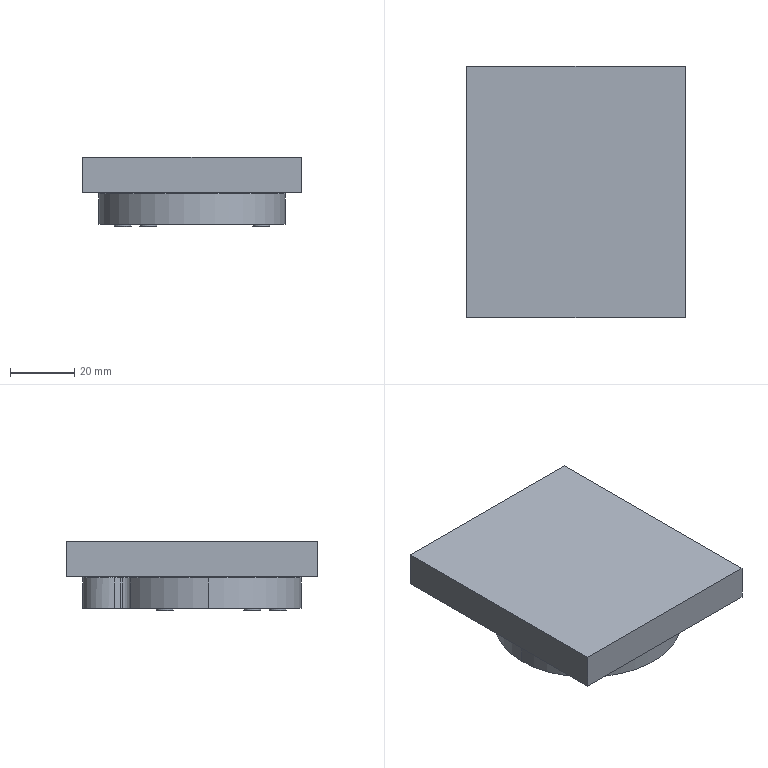NC program | NX | posted with a generic post | part box 68 x 78.27 x 21.8 mm
Lines 751 to 1704 of 10371:
(CAVITY_MILL_COPY_COPY , TOOL : D4)
N1488 T11 M6
N1490 G54
N1492 G17 G0 G90 X-13.811 Y15.944 S9500 M3
N1494 G43 Z30. H11
N1496 Z-0.7
N1498 G94 G1 Z-1.2 F1000.
N1500 X-14.149 Y16.097
N1502 G3 X-15.145 Y15.999 R1.
N1504 X-16.092 Y15.287 R26. F2000.
N1506 G2 X-16.209 Y14.361 R2.5
N1508 G3 X-16.001 Y13.383 R1.
N1510 G1 X-15.879 Y13.247
N1512 Z-0.7
N1514 G0 X-13.811 Y15.944 Z-1.1
N1516 G1 Z-1.6 F1000.
N1518 X-14.149 Y16.097
N1520 G3 X-15.145 Y15.999 R1.
N1522 X-16.092 Y15.287 R26. F2000.
N1524 G2 X-16.209 Y14.361 R2.5
N1526 G3 X-16.001 Y13.383 R1.
N1528 G1 X-15.879 Y13.247
N1530 Z-1.1
N1532 G0 X-13.811 Y15.944 Z-1.5
N1534 G1 Z-2. F1000.
N1536 X-14.149 Y16.097
N1538 G3 X-15.145 Y15.999 R1.
N1540 X-16.092 Y15.287 R26. F2000.
N1542 G2 X-16.209 Y14.361 R2.5
N1544 G3 X-16.001 Y13.383 R1.
N1546 G1 X-15.879 Y13.247
N1548 Z-1.5
N1550 G0 X-13.811 Y15.944 Z-1.9
N1552 G1 Z-2.4 F1000.
N1554 X-14.149 Y16.097
N1556 G3 X-15.145 Y15.999 R1.
N1558 X-16.092 Y15.287 R26. F2000.
N1560 G2 X-16.209 Y14.361 R2.5
N1562 G3 X-16.001 Y13.383 R1.
N1564 G1 X-15.879 Y13.247
N1566 Z-1.9
N1568 G0 X-13.811 Y15.944 Z-2.3
N1570 G1 Z-2.8 F1000.
N1572 X-14.149 Y16.097
N1574 G3 X-15.145 Y15.999 R1.
N1576 X-16.092 Y15.287 R26. F2000.
N1578 G2 X-16.209 Y14.361 R2.5
N1580 G3 X-16.001 Y13.383 R1.
N1582 G1 X-15.879 Y13.247
N1584 Z-2.3
N1586 G0 X-13.811 Y15.944 Z-2.7
N1588 G1 Z-3.2 F1000.
N1590 X-14.149 Y16.097
N1592 G3 X-15.145 Y15.999 R1.
N1594 X-16.092 Y15.287 R26. F2000.
N1596 G2 X-16.209 Y14.361 R2.5
N1598 G3 X-16.001 Y13.383 R1.
N1600 G1 X-15.879 Y13.247
N1602 Z-2.7
N1604 G0 X-13.811 Y15.944 Z-3.1
N1606 G1 Z-3.6 F1000.
N1608 X-14.149 Y16.097
N1610 G3 X-15.145 Y15.999 R1.
N1612 X-16.092 Y15.287 R26. F2000.
N1614 G2 X-16.209 Y14.361 R2.5
N1616 G3 X-16.001 Y13.383 R1.
N1618 G1 X-15.879 Y13.247
N1620 Z-3.1
N1622 G0 X-13.811 Y15.944 Z-3.5
N1624 G1 Z-4. F1000.
N1626 X-14.149 Y16.097
N1628 G3 X-15.145 Y15.999 R1.
N1630 X-16.092 Y15.287 R26. F2000.
N1632 G2 X-16.209 Y14.361 R2.5
N1634 G3 X-16.001 Y13.383 R1.
N1636 G1 X-15.879 Y13.247
N1638 Z-3.5
N1640 G0 X-13.811 Y15.944 Z-3.9
N1642 G1 Z-4.4 F1000.
N1644 X-14.149 Y16.097
N1646 G3 X-15.145 Y15.999 R1.
N1648 X-16.092 Y15.287 R26. F2000.
N1650 G2 X-16.209 Y14.361 R2.5
N1652 G3 X-16.001 Y13.383 R1.
N1654 G1 X-15.879 Y13.247
N1656 Z-3.9
N1658 G0 X-13.811 Y15.944 Z-4.3
N1660 G1 Z-4.8 F1000.
N1662 X-14.149 Y16.097
N1664 G3 X-15.145 Y15.999 R1.
N1666 X-16.092 Y15.287 R26. F2000.
N1668 G2 X-16.209 Y14.361 R2.5
N1670 G3 X-16.001 Y13.383 R1.
N1672 G1 X-15.879 Y13.247
N1674 Z-4.3
N1676 G0 X-13.811 Y15.944 Z-4.7
N1678 G1 Z-5.2 F1000.
N1680 X-14.149 Y16.097
N1682 G3 X-15.145 Y15.999 R1.
N1684 X-16.092 Y15.287 R26. F2000.
N1686 G2 X-16.209 Y14.361 R2.5
N1688 G3 X-16.001 Y13.383 R1.
N1690 G1 X-15.879 Y13.247
N1692 Z-4.7
N1694 G0 X-13.811 Y15.944 Z-5.1
N1696 G1 Z-5.6 F1000.
N1698 X-14.149 Y16.097
N1700 G3 X-15.145 Y15.999 R1.
N1702 X-16.092 Y15.287 R26. F2000.
N1704 G2 X-16.209 Y14.361 R2.5
N1706 G3 X-16.001 Y13.383 R1.
N1708 G1 X-15.879 Y13.247
N1710 Z-5.1
N1712 G0 X-13.811 Y15.944 Z-5.5
N1714 G1 Z-6. F1000.
N1716 X-14.149 Y16.097
N1718 G3 X-15.145 Y15.999 R1.
N1720 X-16.092 Y15.287 R26. F2000.
N1722 G2 X-16.209 Y14.361 R2.5
N1724 G3 X-16.001 Y13.383 R1.
N1726 G1 X-15.879 Y13.247
N1728 Z-5.5
N1730 G0 X-13.811 Y15.944 Z-5.9
N1732 G1 Z-6.4 F1000.
N1734 X-14.149 Y16.097
N1736 G3 X-15.145 Y15.999 R1.
N1738 X-16.092 Y15.287 R26. F2000.
N1740 G2 X-16.209 Y14.361 R2.5
N1742 G3 X-16.001 Y13.383 R1.
N1744 G1 X-15.879 Y13.247
N1746 Z-5.9
N1748 G0 X-13.811 Y15.944 Z-6.3
N1750 G1 Z-6.8 F1000.
N1752 X-14.149 Y16.097
N1754 G3 X-15.145 Y15.999 R1.
N1756 X-16.092 Y15.287 R26. F2000.
N1758 G2 X-16.209 Y14.361 R2.5
N1760 G3 X-16.001 Y13.383 R1.
N1762 G1 X-15.879 Y13.247
N1764 Z-6.3
N1766 G0 X-13.811 Y15.944 Z-6.7
N1768 G1 Z-7.2 F1000.
N1770 X-14.149 Y16.097
N1772 G3 X-15.145 Y15.999 R1.
N1774 X-16.092 Y15.287 R26. F2000.
N1776 G2 X-16.209 Y14.361 R2.5
N1778 G3 X-16.001 Y13.383 R1.
N1780 G1 X-15.879 Y13.247
N1782 Z-6.7
N1784 G0 X-13.811 Y15.944 Z-7.1
N1786 G1 Z-7.6 F1000.
N1788 X-14.149 Y16.097
N1790 G3 X-15.145 Y15.999 R1.
N1792 X-16.092 Y15.287 R26. F2000.
N1794 G2 X-16.209 Y14.361 R2.5
N1796 G3 X-16.001 Y13.383 R1.
N1798 G1 X-15.879 Y13.247
N1800 Z-7.1
N1802 G0 X-13.811 Y15.944 Z-7.5
N1804 G1 Z-8. F1000.
N1806 X-14.149 Y16.097
N1808 G3 X-15.145 Y15.999 R1.
N1810 X-16.092 Y15.287 R26. F2000.
N1812 G2 X-16.209 Y14.361 R2.5
N1814 G3 X-16.001 Y13.383 R1.
N1816 G1 X-15.879 Y13.247
N1818 Z-7.5
N1820 G0 X-13.811 Y15.944 Z-7.9
N1822 G1 Z-8.4 F1000.
N1824 X-14.149 Y16.097
N1826 G3 X-15.145 Y15.999 R1.
N1828 X-16.092 Y15.287 R26. F2000.
N1830 G2 X-16.209 Y14.361 R2.5
N1832 G3 X-16.001 Y13.383 R1.
N1834 G1 X-15.879 Y13.247
N1836 Z-7.9
N1838 G0 X-13.811 Y15.944 Z-8.3
N1840 G1 Z-8.8 F1000.
N1842 X-14.149 Y16.097
N1844 G3 X-15.145 Y15.999 R1.
N1846 X-16.092 Y15.287 R26. F2000.
N1848 G2 X-16.209 Y14.361 R2.5
N1850 G3 X-16.001 Y13.383 R1.
N1852 G1 X-15.879 Y13.247
N1854 Z-8.3
N1856 G0 X-12.092 Y16.975 Z-8.633
N1858 G1 Z-9.133 F1000.
N1860 X-12.417 Y17.154
N1862 G3 X-13.417 Y17.136 R1.
N1864 X-15.863 Y15.465 R26. F2000.
N1866 G1 X-14.342 Y13.096
N1868 G3 X-13.453 Y12.637 R1.
N1870 G1 X-13.107 Y12.654
N1872 Z-8.633
N1874 G0 X-12.092 Y16.975 Z-8.967
N1876 G1 Z-9.467 F1000.
N1878 X-12.417 Y17.154
N1880 G3 X-13.417 Y17.136 R1.
N1882 X-15.863 Y15.465 R26. F2000.
N1884 G1 X-14.342 Y13.096
N1886 G3 X-13.453 Y12.637 R1.
N1888 G1 X-13.107 Y12.654
N1890 Z-8.967
N1892 G0 X-12.092 Y16.975 Z-9.3
N1894 G1 Z-9.8 F1000.
N1896 X-12.417 Y17.154
N1898 G3 X-13.417 Y17.136 R1.
N1900 X-15.863 Y15.465 R26. F2000.
N1902 G1 X-14.342 Y13.096
N1904 G3 X-13.453 Y12.637 R1.
N1906 G1 X-13.107 Y12.654
N1908 Z-9.3
N1910 G0 Z-5.8
N1912 X-10.957 Y9.306
N1914 Z-8.633
N1916 G1 Z-9.133 F1000.
N1918 X-11.116 Y8.998
N1920 G3 X-11.069 Y7.999 R1.
N1922 G1 X-9.482 Y5.528 F2000.
N1924 X-7.032 Y7.148
N1926 G3 X-6.585 Y8.042 R1.
N1928 G1 X-6.606 Y8.388
N1930 Z-8.633
N1932 G0 X-10.957 Y9.306 Z-8.967
N1934 G1 Z-9.467 F1000.
N1936 X-11.116 Y8.998
N1938 G3 X-11.069 Y7.999 R1.
N1940 G1 X-9.482 Y5.528 F2000.
N1942 X-7.032 Y7.148
N1944 G3 X-6.585 Y8.042 R1.
N1946 G1 X-6.606 Y8.388
N1948 Z-8.967
N1950 G0 X-10.957 Y9.306 Z-9.3
N1952 G1 Z-9.8 F1000.
N1954 X-11.116 Y8.998
N1956 G3 X-11.069 Y7.999 R1.
N1958 G1 X-9.482 Y5.528 F2000.
N1960 X-7.032 Y7.148
N1962 G3 X-6.585 Y8.042 R1.
N1964 G1 X-6.606 Y8.388
N1966 Z-9.3
N1968 G0 Z30.
N1970 X2.622 Y23.856
N1972 Z-0.7
N1974 G1 Z-1.2 F1000.
N1976 X2.46 Y23.94
N1978 G3 X1.461 Y23.895 R1.
N1980 G2 X0.853 Y23.614 R2.5 F2000.
N1982 X0.471 Y23.021 R6.
N1984 G3 X0.363 Y22.027 R1.
N1986 G1 X0.468 Y21.788
N1988 Z-0.7
N1990 G0 X2.622 Y23.856 Z-1.1
N1992 G1 Z-1.6 F1000.
N1994 X2.46 Y23.94
N1996 G3 X1.461 Y23.895 R1.
N1998 G2 X0.853 Y23.614 R2.5 F2000.
N2000 X0.471 Y23.021 R6.
N2002 G3 X0.363 Y22.027 R1.
N2004 G1 X0.468 Y21.788
N2006 Z-1.1
N2008 G0 X2.622 Y23.856 Z-1.5
N2010 G1 Z-2. F1000.
N2012 X2.46 Y23.94
N2014 G3 X1.461 Y23.895 R1.
N2016 G2 X0.853 Y23.614 R2.5 F2000.
N2018 X0.471 Y23.021 R6.
N2020 G3 X0.363 Y22.027 R1.
N2022 G1 X0.468 Y21.788
N2024 Z-1.5
N2026 G0 X2.622 Y23.856 Z-1.9
N2028 G1 Z-2.4 F1000.
N2030 X2.46 Y23.94
N2032 G3 X1.461 Y23.895 R1.
N2034 G2 X0.853 Y23.614 R2.5 F2000.
N2036 X0.471 Y23.021 R6.
N2038 G3 X0.363 Y22.027 R1.
N2040 G1 X0.468 Y21.788
N2042 Z-1.9
N2044 G0 X2.622 Y23.856 Z-2.3
N2046 G1 Z-2.8 F1000.
N2048 X2.46 Y23.94
N2050 G3 X1.461 Y23.895 R1.
N2052 G2 X0.853 Y23.614 R2.5 F2000.
N2054 X0.471 Y23.021 R6.
N2056 G3 X0.363 Y22.027 R1.
N2058 G1 X0.468 Y21.788
N2060 Z-2.3
N2062 G0 X2.622 Y23.856 Z-2.7
N2064 G1 Z-3.2 F1000.
N2066 X2.46 Y23.94
N2068 G3 X1.461 Y23.895 R1.
N2070 G2 X0.853 Y23.614 R2.5 F2000.
N2072 X0.471 Y23.021 R6.
N2074 G3 X0.363 Y22.027 R1.
N2076 G1 X0.468 Y21.788
N2078 Z-2.7
N2080 G0 X2.622 Y23.856 Z-3.1
N2082 G1 Z-3.6 F1000.
N2084 X2.46 Y23.94
N2086 G3 X1.461 Y23.895 R1.
N2088 G2 X0.853 Y23.614 R2.5 F2000.
N2090 X0.471 Y23.021 R6.
N2092 G3 X0.363 Y22.027 R1.
N2094 G1 X0.468 Y21.788
N2096 Z-3.1
N2098 G0 X2.622 Y23.856 Z-3.5
N2100 G1 Z-4. F1000.
N2102 X2.46 Y23.94
N2104 G3 X1.461 Y23.895 R1.
N2106 G2 X0.853 Y23.614 R2.5 F2000.
N2108 X0.471 Y23.021 R6.
N2110 G3 X0.363 Y22.027 R1.
N2112 G1 X0.468 Y21.788
N2114 Z-3.5
N2116 G0 X2.622 Y23.856 Z-3.9
N2118 G1 Z-4.4 F1000.
N2120 X2.46 Y23.94
N2122 G3 X1.461 Y23.895 R1.
N2124 G2 X0.853 Y23.614 R2.5 F2000.
N2126 X0.471 Y23.021 R6.
N2128 G3 X0.363 Y22.027 R1.
N2130 G1 X0.468 Y21.788
N2132 Z-3.9
N2134 G0 X2.622 Y23.856 Z-4.3
N2136 G1 Z-4.8 F1000.
N2138 X2.46 Y23.94
N2140 G3 X1.461 Y23.895 R1.
N2142 G2 X0.853 Y23.614 R2.5 F2000.
N2144 X0.471 Y23.021 R6.
N2146 G3 X0.363 Y22.027 R1.
N2148 G1 X0.468 Y21.788
N2150 Z-4.3
N2152 G0 X2.622 Y23.856 Z-4.7
N2154 G1 Z-5.2 F1000.
N2156 X2.46 Y23.94
N2158 G3 X1.461 Y23.895 R1.
N2160 G2 X0.853 Y23.614 R2.5 F2000.
N2162 X0.471 Y23.021 R6.
N2164 G3 X0.363 Y22.027 R1.
N2166 G1 X0.468 Y21.788
N2168 Z-4.7
N2170 G0 X2.622 Y23.856 Z-5.1
N2172 G1 Z-5.6 F1000.
N2174 X2.46 Y23.94
N2176 G3 X1.461 Y23.895 R1.
N2178 G2 X0.853 Y23.614 R2.5 F2000.
N2180 X0.471 Y23.021 R6.
N2182 G3 X0.363 Y22.027 R1.
N2184 G1 X0.468 Y21.788
N2186 Z-5.1
N2188 G0 X2.622 Y23.856 Z-5.5
N2190 G1 Z-6. F1000.
N2192 X2.46 Y23.94
N2194 G3 X1.461 Y23.895 R1.
N2196 G2 X0.853 Y23.614 R2.5 F2000.
N2198 X0.471 Y23.021 R6.
N2200 G3 X0.363 Y22.027 R1.
N2202 G1 X0.468 Y21.788
N2204 Z-5.5
N2206 G0 X2.622 Y23.856 Z-5.9
N2208 G1 Z-6.4 F1000.
N2210 X2.46 Y23.94
N2212 G3 X1.461 Y23.895 R1.
N2214 G2 X0.853 Y23.614 R2.5 F2000.
N2216 X0.471 Y23.021 R6.
N2218 G3 X0.363 Y22.027 R1.
N2220 G1 X0.468 Y21.788
N2222 Z-5.9
N2224 G0 X2.622 Y23.856 Z-6.3
N2226 G1 Z-6.8 F1000.
N2228 X2.46 Y23.94
N2230 G3 X1.461 Y23.895 R1.
N2232 G2 X0.853 Y23.614 R2.5 F2000.
N2234 X0.471 Y23.021 R6.
N2236 G3 X0.363 Y22.027 R1.
N2238 G1 X0.468 Y21.788
N2240 Z-6.3
N2242 G0 X2.622 Y23.856 Z-6.7
N2244 G1 Z-7.2 F1000.
N2246 X2.46 Y23.94
N2248 G3 X1.461 Y23.895 R1.
N2250 G2 X0.853 Y23.614 R2.5 F2000.
N2252 X0.471 Y23.021 R6.
N2254 G3 X0.363 Y22.027 R1.
N2256 G1 X0.468 Y21.788
N2258 Z-6.7
N2260 G0 X2.622 Y23.856 Z-7.1
N2262 G1 Z-7.6 F1000.
N2264 X2.46 Y23.94
N2266 G3 X1.461 Y23.895 R1.
N2268 G2 X0.853 Y23.614 R2.5 F2000.
N2270 X0.471 Y23.021 R6.
N2272 G3 X0.363 Y22.027 R1.
N2274 G1 X0.468 Y21.788
N2276 Z-7.1
N2278 G0 X2.622 Y23.856 Z-7.5
N2280 G1 Z-8. F1000.
N2282 X2.46 Y23.94
N2284 G3 X1.461 Y23.895 R1.
N2286 G2 X0.853 Y23.614 R2.5 F2000.
N2288 X0.471 Y23.021 R6.
N2290 G3 X0.363 Y22.027 R1.
N2292 G1 X0.468 Y21.788
N2294 Z-7.5
N2296 G0 X2.622 Y23.856 Z-7.9
N2298 G1 Z-8.4 F1000.
N2300 X2.46 Y23.94
N2302 G3 X1.461 Y23.895 R1.
N2304 G2 X0.853 Y23.614 R2.5 F2000.
N2306 X0.471 Y23.021 R6.
N2308 G3 X0.363 Y22.027 R1.
N2310 G1 X0.468 Y21.788
N2312 Z-7.9
N2314 G0 X2.622 Y23.856 Z-8.3
N2316 G1 Z-8.8 F1000.
N2318 X2.46 Y23.94
N2320 G3 X1.461 Y23.895 R1.
N2322 G2 X0.853 Y23.614 R2.5 F2000.
N2324 X0.471 Y23.021 R6.
N2326 G3 X0.363 Y22.027 R1.
N2328 G1 X0.468 Y21.788
N2330 Z-8.3
N2332 G0 X3.225 Y21.978 Z-8.633
N2334 G1 Z-9.133 F1000.
N2336 X3.122 Y22.309
N2338 G3 X2.387 Y22.988 R1.
N2340 G1 X0.706 Y23.368 F2000.
N2342 G2 X-0.245 Y22.209 R6.
N2344 G3 X-0.53 Y21.251 R1.
N2346 G1 X-0.469 Y20.996
N2348 Z-8.633
N2350 G0 X3.225 Y21.978 Z-8.967
N2352 G1 Z-9.467 F1000.
N2354 X3.122 Y22.309
N2356 G3 X2.387 Y22.988 R1.
N2358 G1 X0.706 Y23.368 F2000.
N2360 G2 X-0.245 Y22.209 R6.
N2362 G3 X-0.53 Y21.251 R1.
N2364 G1 X-0.469 Y20.996
N2366 Z-8.967
N2368 G0 X3.225 Y21.978 Z-9.3
N2370 G1 Z-9.8 F1000.
N2372 X3.122 Y22.309
N2374 G3 X2.387 Y22.988 R1.
N2376 G1 X0.706 Y23.368 F2000.
N2378 G2 X-0.245 Y22.209 R6.
N2380 G3 X-0.53 Y21.251 R1.
N2382 G1 X-0.469 Y20.996
N2384 Z-9.3
N2386 G0 Z-5.8
N2388 X6.139 Y16.811
N2390 Z-8.633
N2392 G1 Z-9.133 F1000.
N2394 X6.448 Y16.656
N2396 G3 X7.447 Y16.716 R1.
N2398 G1 X10.699 Y18.865 F2000.
N2400 Y20.3
N2402 G2 X10.592 Y21.134 R7.
N2404 G1 X6.468 Y22.066
N2406 G3 X5.513 Y21.769 R1.
N2408 G1 X5.278 Y21.514
N2410 Z-8.633
N2412 G0 X6.139 Y16.811 Z-8.967
N2414 G1 Z-9.467 F1000.
N2416 X6.448 Y16.656
N2418 G3 X7.447 Y16.716 R1.
N2420 G1 X10.699 Y18.865 F2000.
N2422 Y20.3
N2424 G2 X10.592 Y21.134 R7.
N2426 G1 X6.468 Y22.066
N2428 G3 X5.513 Y21.769 R1.
N2430 G1 X5.278 Y21.514
N2432 Z-8.967
N2434 G0 X6.139 Y16.811 Z-9.3
N2436 G1 Z-9.8 F1000.
N2438 X6.448 Y16.656
N2440 G3 X7.447 Y16.716 R1.
N2442 G1 X10.699 Y18.865 F2000.
N2444 Y20.3
N2446 G2 X10.592 Y21.134 R7.
N2448 G1 X6.468 Y22.066
N2450 G3 X5.513 Y21.769 R1.
N2452 G1 X5.278 Y21.514
N2454 Z-9.3
N2456 G0 Z30.
N2458 X14.615 Y10.721
N2460 Z-0.7
N2462 G1 Z-1.2 F1000.
N2464 X14.881 Y10.741
N2466 G3 X15.708 Y11.303 R1.
N2468 G2 X17.045 Y13.153 R6.5 F2000.
N2470 G3 X14.895 Y14.943 R25.
N2472 X13.902 Y15.058 R1.
N2474 G1 X13.56 Y14.91
N2476 Z-0.7
N2478 G0 X14.615 Y10.721 Z-1.1
N2480 G1 Z-1.6 F1000.
N2482 X14.881 Y10.741
N2484 G3 X15.708 Y11.303 R1.
N2486 G2 X17.045 Y13.153 R6.5 F2000.
N2488 G3 X14.895 Y14.943 R25.
N2490 X13.902 Y15.058 R1.
N2492 G1 X13.56 Y14.91
N2494 Z-1.1
N2496 G0 X14.615 Y10.721 Z-1.5
N2498 G1 Z-2. F1000.
N2500 X14.881 Y10.741
N2502 G3 X15.708 Y11.303 R1.
N2504 G2 X17.045 Y13.153 R6.5 F2000.
N2506 G3 X14.895 Y14.943 R25.
N2508 X13.902 Y15.058 R1.
N2510 G1 X13.56 Y14.91
N2512 Z-1.5
N2514 G0 X14.615 Y10.721 Z-1.9
N2516 G1 Z-2.4 F1000.
N2518 X14.881 Y10.741
N2520 G3 X15.708 Y11.303 R1.
N2522 G2 X17.045 Y13.153 R6.5 F2000.
N2524 G3 X14.895 Y14.943 R25.
N2526 X13.902 Y15.058 R1.
N2528 G1 X13.56 Y14.91
N2530 Z-1.9
N2532 G0 X14.615 Y10.721 Z-2.3
N2534 G1 Z-2.8 F1000.
N2536 X14.881 Y10.741
N2538 G3 X15.708 Y11.303 R1.
N2540 G2 X17.045 Y13.153 R6.5 F2000.
N2542 G3 X14.895 Y14.943 R25.
N2544 X13.902 Y15.058 R1.
N2546 G1 X13.56 Y14.91
N2548 Z-2.3
N2550 G0 X14.615 Y10.721 Z-2.7
N2552 G1 Z-3.2 F1000.
N2554 X14.881 Y10.741
N2556 G3 X15.708 Y11.303 R1.
N2558 G2 X17.045 Y13.153 R6.5 F2000.
N2560 G3 X14.895 Y14.943 R25.
N2562 X13.902 Y15.058 R1.
N2564 G1 X13.56 Y14.91
N2566 Z-2.7
N2568 G0 X14.615 Y10.721 Z-3.1
N2570 G1 Z-3.6 F1000.
N2572 X14.881 Y10.741
N2574 G3 X15.708 Y11.303 R1.
N2576 G2 X17.045 Y13.153 R6.5 F2000.
N2578 G3 X14.895 Y14.943 R25.
N2580 X13.902 Y15.058 R1.
N2582 G1 X13.56 Y14.91
N2584 Z-3.1
N2586 G0 X14.615 Y10.721 Z-3.5
N2588 G1 Z-4. F1000.
N2590 X14.881 Y10.741
N2592 G3 X15.708 Y11.303 R1.
N2594 G2 X17.045 Y13.153 R6.5 F2000.
N2596 G3 X14.895 Y14.943 R25.
N2598 X13.902 Y15.058 R1.
N2600 G1 X13.56 Y14.91
N2602 Z-3.5
N2604 G0 X14.615 Y10.721 Z-3.9
N2606 G1 Z-4.4 F1000.
N2608 X14.881 Y10.741
N2610 G3 X15.708 Y11.303 R1.
N2612 G2 X17.045 Y13.153 R6.5 F2000.
N2614 G3 X14.895 Y14.943 R25.
N2616 X13.902 Y15.058 R1.
N2618 G1 X13.56 Y14.91
N2620 Z-3.9
N2622 G0 X14.615 Y10.721 Z-4.3
N2624 G1 Z-4.8 F1000.
N2626 X14.881 Y10.741
N2628 G3 X15.708 Y11.303 R1.
N2630 G2 X17.045 Y13.153 R6.5 F2000.
N2632 G3 X14.895 Y14.943 R25.
N2634 X13.902 Y15.058 R1.
N2636 G1 X13.56 Y14.91
N2638 Z-4.3
N2640 G0 X14.615 Y10.721 Z-4.7
N2642 G1 Z-5.2 F1000.
N2644 X14.881 Y10.741
N2646 G3 X15.708 Y11.303 R1.
N2648 G2 X17.045 Y13.153 R6.5 F2000.
N2650 G3 X14.895 Y14.943 R25.
N2652 X13.902 Y15.058 R1.
N2654 G1 X13.56 Y14.91
N2656 Z-4.7
N2658 G0 X14.615 Y10.721 Z-5.1
N2660 G1 Z-5.6 F1000.
N2662 X14.881 Y10.741
N2664 G3 X15.708 Y11.303 R1.
N2666 G2 X17.045 Y13.153 R6.5 F2000.
N2668 G3 X14.895 Y14.943 R25.
N2670 X13.902 Y15.058 R1.
N2672 G1 X13.56 Y14.91
N2674 Z-5.1
N2676 G0 X14.615 Y10.721 Z-5.5
N2678 G1 Z-6. F1000.
N2680 X14.881 Y10.741
N2682 G3 X15.708 Y11.303 R1.
N2684 G2 X17.045 Y13.153 R6.5 F2000.
N2686 G3 X14.895 Y14.943 R25.
N2688 X13.902 Y15.058 R1.
N2690 G1 X13.56 Y14.91
N2692 Z-5.5
N2694 G0 X14.615 Y10.721 Z-5.9
N2696 G1 Z-6.4 F1000.
N2698 X14.881 Y10.741
N2700 G3 X15.708 Y11.303 R1.
N2702 G2 X17.045 Y13.153 R6.5 F2000.
N2704 G3 X14.895 Y14.943 R25.
N2706 X13.902 Y15.058 R1.
N2708 G1 X13.56 Y14.91
N2710 Z-5.9
N2712 G0 X14.615 Y10.721 Z-6.3
N2714 G1 Z-6.8 F1000.
N2716 X14.881 Y10.741
N2718 G3 X15.708 Y11.303 R1.
N2720 G2 X17.045 Y13.153 R6.5 F2000.
N2722 G3 X14.895 Y14.943 R25.
N2724 X13.902 Y15.058 R1.
N2726 G1 X13.56 Y14.91
N2728 Z-6.3
N2730 G0 X14.615 Y10.721 Z-6.7
N2732 G1 Z-7.2 F1000.
N2734 X14.881 Y10.741
N2736 G3 X15.708 Y11.303 R1.
N2738 G2 X17.045 Y13.153 R6.5 F2000.
N2740 G3 X14.895 Y14.943 R25.
N2742 X13.902 Y15.058 R1.
N2744 G1 X13.56 Y14.91
N2746 Z-6.7
N2748 G0 X14.615 Y10.721 Z-7.1
N2750 G1 Z-7.6 F1000.
N2752 X14.881 Y10.741
N2754 G3 X15.708 Y11.303 R1.
N2756 G2 X17.045 Y13.153 R6.5 F2000.
N2758 G3 X14.895 Y14.943 R25.
N2760 X13.902 Y15.058 R1.
N2762 G1 X13.56 Y14.91
N2764 Z-7.1
N2766 G0 X14.615 Y10.721 Z-7.5
N2768 G1 Z-8. F1000.
N2770 X14.881 Y10.741
N2772 G3 X15.708 Y11.303 R1.
N2774 G2 X17.045 Y13.153 R6.5 F2000.
N2776 G3 X14.895 Y14.943 R25.
N2778 X13.902 Y15.058 R1.
N2780 G1 X13.56 Y14.91
N2782 Z-7.5
N2784 G0 X14.615 Y10.721 Z-7.9
N2786 G1 Z-8.4 F1000.
N2788 X14.881 Y10.741
N2790 G3 X15.708 Y11.303 R1.
N2792 G2 X17.045 Y13.153 R6.5 F2000.
N2794 G3 X14.895 Y14.943 R25.
N2796 X13.902 Y15.058 R1.
N2798 G1 X13.56 Y14.91
N2800 Z-7.9
N2802 G0 X14.615 Y10.721 Z-8.3
N2804 G1 Z-8.8 F1000.
N2806 X14.881 Y10.741
N2808 G3 X15.708 Y11.303 R1.
N2810 G2 X17.045 Y13.153 R6.5 F2000.
N2812 G3 X14.895 Y14.943 R25.
N2814 X13.902 Y15.058 R1.
N2816 G1 X13.56 Y14.91
N2818 Z-8.3
N2820 G0 Z30.
N2822 X23.927 Y-1.511
N2824 Z-0.7
N2826 G1 Z-1.2 F1000.
N2828 X24.208 Y-1.266
N2830 G3 X24.532 Y-0.32 R1.
N2832 X23.84 Y2.391 R25. F2000.
N2834 G2 X21.595 Y1.979 R6.5
N2836 G3 X20.731 Y1.475 R1.
N2838 G1 X20.599 Y1.243
N2840 Z-0.7
N2842 G0 X23.927 Y-1.511 Z-1.1
N2844 G1 Z-1.6 F1000.
N2846 X24.208 Y-1.266
N2848 G3 X24.532 Y-0.32 R1.
N2850 X23.84 Y2.391 R25. F2000.
N2852 G2 X21.595 Y1.979 R6.5
N2854 G3 X20.731 Y1.475 R1.
N2856 G1 X20.599 Y1.243
N2858 Z-1.1
N2860 G0 X23.927 Y-1.511 Z-1.5
N2862 G1 Z-2. F1000.
N2864 X24.208 Y-1.266
N2866 G3 X24.532 Y-0.32 R1.
N2868 X23.84 Y2.391 R25. F2000.
N2870 G2 X21.594 Y1.979 R6.5
N2872 G3 X20.731 Y1.475 R1.
N2874 G1 X20.599 Y1.243
N2876 Z-1.5
N2878 G0 X23.927 Y-1.511 Z-1.9
N2880 G1 Z-2.4 F1000.
N2882 X24.208 Y-1.266
N2884 G3 X24.532 Y-0.32 R1.
N2886 X23.84 Y2.391 R25. F2000.
N2888 G2 X21.594 Y1.979 R6.5
N2890 G3 X20.731 Y1.475 R1.
N2892 G1 X20.598 Y1.243
N2894 Z-1.9
N2896 G0 X23.927 Y-1.511 Z-2.3
N2898 G1 Z-2.8 F1000.
N2900 X24.208 Y-1.266
N2902 G3 X24.532 Y-0.32 R1.
N2904 X23.84 Y2.391 R25. F2000.
N2906 G2 X21.594 Y1.979 R6.5
N2908 G3 X20.73 Y1.475 R1.
N2910 G1 X20.598 Y1.243
N2912 Z-2.3
N2914 G0 X23.927 Y-1.511 Z-2.7
N2916 G1 Z-3.2 F1000.
N2918 X24.208 Y-1.266
N2920 G3 X24.532 Y-0.32 R1.
N2922 X23.84 Y2.391 R25. F2000.
N2924 G2 X21.595 Y1.979 R6.5
N2926 G3 X20.731 Y1.475 R1.
N2928 G1 X20.599 Y1.243
N2930 Z-2.7
N2932 G0 X23.927 Y-1.511 Z-3.1
N2934 G1 Z-3.6 F1000.
N2936 X24.208 Y-1.266
N2938 G3 X24.532 Y-0.32 R1.
N2940 X23.84 Y2.391 R25. F2000.
N2942 G2 X21.595 Y1.979 R6.5
N2944 G3 X20.731 Y1.475 R1.
N2946 G1 X20.599 Y1.243
N2948 Z-3.1
N2950 G0 X23.927 Y-1.512 Z-3.5
N2952 G1 Z-4. F1000.
N2954 X24.208 Y-1.266
N2956 G3 X24.532 Y-0.32 R1.
N2958 X23.84 Y2.391 R25. F2000.
N2960 G2 X21.595 Y1.979 R6.5
N2962 G3 X20.731 Y1.475 R1.
N2964 G1 X20.599 Y1.243
N2966 Z-3.5
N2968 G0 X23.927 Y-1.512 Z-3.9
N2970 G1 Z-4.4 F1000.
N2972 X24.208 Y-1.266
N2974 G3 X24.532 Y-0.32 R1.
N2976 X23.84 Y2.391 R25. F2000.
N2978 G2 X21.595 Y1.979 R6.5
N2980 G3 X20.731 Y1.475 R1.
N2982 G1 X20.599 Y1.243
N2984 Z-3.9
N2986 G0 X23.927 Y-1.512 Z-4.3
N2988 G1 Z-4.8 F1000.
N2990 X24.208 Y-1.267
N2992 G3 X24.532 Y-0.32 R1.
N2994 X23.84 Y2.391 R25. F2000.
N2996 G2 X21.595 Y1.979 R6.5
N2998 G3 X20.731 Y1.475 R1.
N3000 G1 X20.599 Y1.243
N3002 Z-4.3
N3004 G0 X23.927 Y-1.512 Z-4.7
N3006 G1 Z-5.2 F1000.
N3008 X24.208 Y-1.267
N3010 G3 X24.532 Y-0.32 R1.
N3012 X23.84 Y2.391 R25. F2000.
N3014 G2 X21.595 Y1.979 R6.5
N3016 G3 X20.731 Y1.475 R1.
N3018 G1 X20.599 Y1.243
N3020 Z-4.7
N3022 G0 X23.927 Y-1.512 Z-5.1
N3024 G1 Z-5.6 F1000.
N3026 X24.208 Y-1.267
N3028 G3 X24.532 Y-0.321 R1.
N3030 X23.84 Y2.391 R25. F2000.
N3032 G2 X21.595 Y1.979 R6.5
N3034 G3 X20.731 Y1.475 R1.
N3036 G1 X20.599 Y1.243
N3038 Z-5.1
N3040 G0 X23.927 Y-1.512 Z-5.5
N3042 G1 Z-6. F1000.
N3044 X24.208 Y-1.267
N3046 G3 X24.532 Y-0.321 R1.
N3048 X23.84 Y2.391 R25. F2000.
N3050 G2 X21.595 Y1.979 R6.5
N3052 G3 X20.731 Y1.475 R1.
N3054 G1 X20.599 Y1.243
N3056 Z-5.5
N3058 G0 X23.927 Y-1.512 Z-5.9
N3060 G1 Z-6.4 F1000.
N3062 X24.208 Y-1.267
N3064 G3 X24.532 Y-0.321 R1.
N3066 X23.84 Y2.391 R25. F2000.
N3068 G2 X21.594 Y1.979 R6.5
N3070 G3 X20.731 Y1.475 R1.
N3072 G1 X20.599 Y1.243
N3074 Z-5.9
N3076 G0 X23.927 Y-1.512 Z-6.3
N3078 G1 Z-6.8 F1000.
N3080 X24.208 Y-1.267
N3082 G3 X24.532 Y-0.321 R1.
N3084 X23.84 Y2.391 R25. F2000.
N3086 G2 X21.594 Y1.979 R6.5
N3088 G3 X20.731 Y1.475 R1.
N3090 G1 X20.599 Y1.243
N3092 Z-6.3
N3094 G0 X23.927 Y-1.512 Z-6.7
N3096 G1 Z-7.2 F1000.
N3098 X24.208 Y-1.267
N3100 G3 X24.532 Y-0.321 R1.
N3102 X23.84 Y2.391 R25. F2000.
N3104 G2 X21.594 Y1.979 R6.5
N3106 G3 X20.731 Y1.475 R1.
N3108 G1 X20.599 Y1.243
N3110 Z-6.7
N3112 G0 X23.927 Y-1.512 Z-7.1
N3114 G1 Z-7.6 F1000.
N3116 X24.208 Y-1.267
N3118 G3 X24.532 Y-0.321 R1.
N3120 X23.84 Y2.391 R25. F2000.
N3122 G2 X21.594 Y1.979 R6.5
N3124 G3 X20.731 Y1.475 R1.
N3126 G1 X20.599 Y1.243
N3128 Z-7.1
N3130 G0 X23.927 Y-1.512 Z-7.5
N3132 G1 Z-8. F1000.
N3134 X24.208 Y-1.267
N3136 G3 X24.532 Y-0.321 R1.
N3138 X23.84 Y2.391 R25. F2000.
N3140 G2 X21.594 Y1.979 R6.5
N3142 G3 X20.731 Y1.475 R1.
N3144 G1 X20.598 Y1.243
N3146 Z-7.5
N3148 G0 X23.927 Y-1.512 Z-7.9
N3150 G1 Z-8.4 F1000.
N3152 X24.208 Y-1.267
N3154 G3 X24.532 Y-0.321 R1.
N3156 X23.84 Y2.391 R25. F2000.
N3158 G2 X21.594 Y1.979 R6.5
N3160 G3 X20.731 Y1.475 R1.
N3162 G1 X20.598 Y1.243
N3164 Z-7.9
N3166 G0 X23.927 Y-1.512 Z-8.3
N3168 G1 Z-8.8 F1000.
N3170 X24.208 Y-1.267
N3172 G3 X24.532 Y-0.321 R1.
N3174 X23.84 Y2.391 R25. F2000.
N3176 G2 X21.594 Y1.979 R6.5
N3178 G3 X20.731 Y1.475 R1.
N3180 G1 X20.598 Y1.243
N3182 Z-8.3
N3184 G0 Z-5.4
N3186 X4.717 Y-3.618
N3188 Z-8.633
N3190 G1 Z-9.133 F1000.
N3192 X4.957 Y-3.188
N3194 G3 X4.943 Y-2.188 R1.
N3196 X3.95 Y-0.95 R5.755 F2000.
N3198 G1 X3.88 Y-0.87
N3200 X3.775 Y-0.88
N3202 X2.555
N3204 G3 X1.689 Y-1.38 R1.
N3206 G1 X1.516 Y-1.68
N3208 Z-8.633
N3210 G0 X4.598 Y-3.914 Z-8.967
N3212 G1 Z-9.467 F1000.
N3214 X4.859 Y-3.488
N3216 G3 X4.887 Y-2.489 R1.
N3218 X3.814 Y-1.093 R5.557 F2000.
N3220 G1 X3.775 Y-1.078
N3222 X2.431
N3224 G3 X1.565 Y-1.578 R1.
N3226 G1 X1.392 Y-1.878
N3228 Z-8.967
N3230 G0 X4.563 Y-4.004 Z-9.3
N3232 G1 Z-9.8 F1000.
N3234 X4.832 Y-3.58
N3236 G3 X4.873 Y-2.581 R1.
N3238 X3.778 Y-1.136 R5.501 F2000.
N3240 G1 X2.392 Y-1.134
N3242 G3 X1.526 Y-1.634 R1.
N3244 G1 X1.353 Y-1.934
N3246 Z-9.3
N3248 G0 Z-5.8
N3250 X-1.516 Y-1.68
N3252 Z-8.633
N3254 G1 Z-9.133 F1000.
N3256 X-1.689 Y-1.38
N3258 G3 X-2.555 Y-0.88 R1.
N3260 G1 X-3.775 F2000.
N3262 X-3.88 Y-0.87
N3264 X-3.95 Y-0.95
N3266 G3 X-4.943 Y-2.188 R5.755
N3268 X-4.957 Y-3.188 R1.
N3270 G1 X-4.717 Y-3.618
N3272 Z-8.633
N3274 G0 X-1.392 Y-1.878 Z-8.967
N3276 G1 Z-9.467 F1000.
N3278 X-1.565 Y-1.578
N3280 G3 X-2.431 Y-1.078 R1.
N3282 G1 X-3.775 F2000.
N3284 X-3.814 Y-1.093
N3286 G3 X-4.887 Y-2.489 R5.557
N3288 X-4.859 Y-3.488 R1.
N3290 G1 X-4.598 Y-3.914
N3292 Z-8.967
N3294 G0 X-1.356 Y-1.934 Z-9.3
N3296 G1 Z-9.8 F1000.
N3298 X-1.529 Y-1.634
N3300 G3 X-2.395 Y-1.134 R1.
N3302 G1 X-3.778 Y-1.136 F2000.
N3304 G3 X-4.87 Y-2.577 R5.501
N3306 X-4.83 Y-3.576 R1.
N3308 G1 X-4.562 Y-4.
N3310 Z-9.3
N3312 G0 Z-5.8
N3314 X-4.717 Y-6.652
N3316 Z-8.633
N3318 G1 Z-9.133 F1000.
N3320 X-4.957 Y-7.082
N3322 G3 X-4.943 Y-8.082 R1.
N3324 X-3.95 Y-9.32 R5.755 F2000.
N3326 G1 X-3.88 Y-9.399
N3328 X-3.775 Y-9.389
N3330 X-2.555
N3332 G3 X-1.689 Y-8.889 R1.
N3334 G1 X-1.516 Y-8.589
N3336 Z-8.633
N3338 G0 X-4.598 Y-6.356 Z-8.967
N3340 G1 Z-9.467 F1000.
N3342 X-4.859 Y-6.782
N3344 G3 X-4.887 Y-7.781 R1.
N3346 X-3.814 Y-9.176 R5.557 F2000.
N3348 G1 X-3.775 Y-9.192
N3350 X-2.431
N3352 G3 X-1.565 Y-8.692 R1.
N3354 G1 X-1.392 Y-8.392
N3356 Z-8.967
N3358 G0 X-4.562 Y-6.268 Z-9.3
N3360 G1 Z-9.8 F1000.
N3362 X-4.831 Y-6.692
N3364 G3 X-4.871 Y-7.692 R1.
N3366 X-3.906 Y-9.008 R5.501 F2000.
N3368 G1 X-3.778 Y-9.133
N3370 X-2.393 Y-9.136
N3372 G3 X-1.527 Y-8.636 R1.
N3374 G1 X-1.353 Y-8.336
N3376 Z-9.3
N3378 G0 Z-5.8
N3380 X1.516 Y-8.589
N3382 Z-8.633
N3384 G1 Z-9.133 F1000.
N3386 X1.689 Y-8.889
N3388 G3 X2.555 Y-9.389 R1.